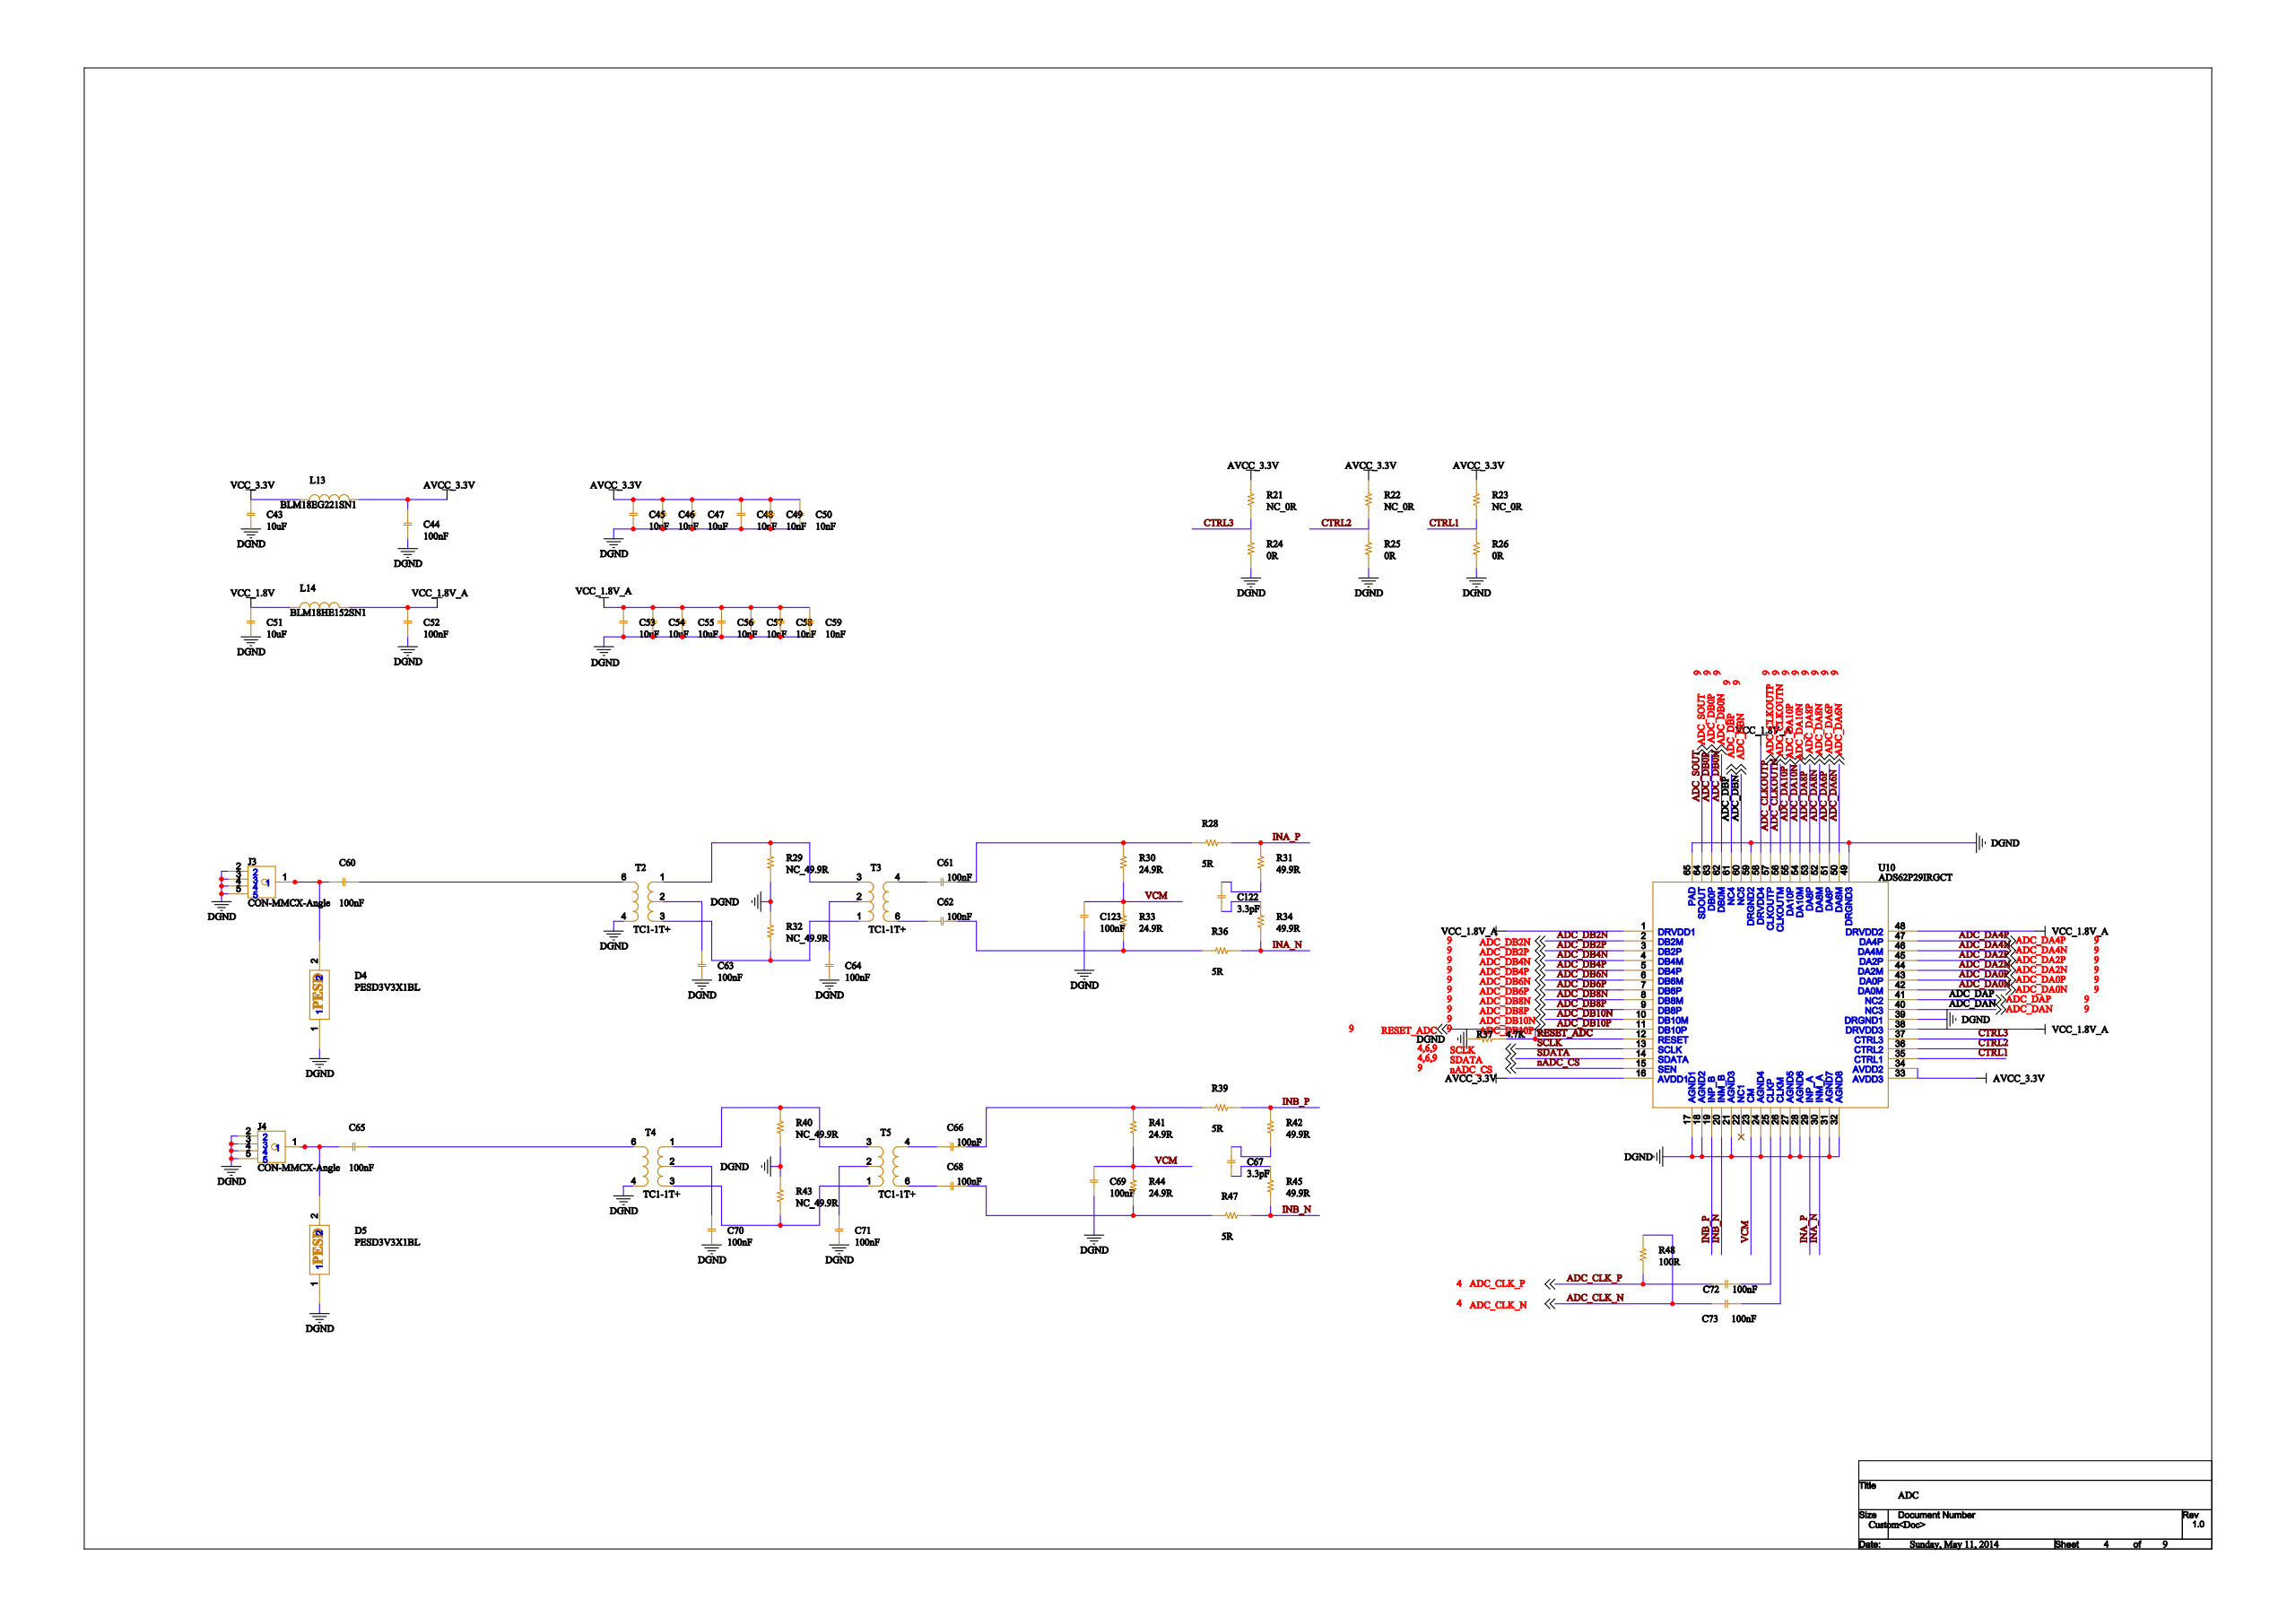Circuit board | Cadence Allegro | 233 parts | 224 nets | one sheet of the schematic
Parts on this sheet (reference | value | footprint):
C43 | 10uF | FPC-0603C
C44 | 100nF | FPC-0402C
C45 | 10uF | FPC-0603C
C46 | 10uF | FPC-0603C
C47 | 10uF | FPC-0603C
C48 | 10nF | FPC-0402C
C49 | 10nF | FPC-0402C
C50 | 10nF | FPC-0402C
C51 | 10uF | FPC-0603C
C52 | 100nF | FPC-0402C
C53 | 10uF | FPC-0603C
C54 | 10uF | FPC-0603C
C55 | 10uF | FPC-0603C
C56 | 10nF | FPC-0402C
C57 | 10nF | FPC-0402C
C58 | 10nF | FPC-0402C
C59 | 10nF | FPC-0402C
C60 | 100nF | FPC-0402C
C61 | 100nF | FPC-0402C
C62 | 100nF | FPC-0402C
C63 | 100nF | FPC-0402C
C64 | 100nF | FPC-0402C
C65 | 100nF | FPC-0402C
C66 | 100nF | FPC-0402C
C67 | 3.3pF | FPC-0402C
C68 | 100nF | FPC-0402C
C69 | 100nF | FPC-0402C
C70 | 100nF | FPC-0402C
C71 | 100nF | FPC-0402C
C72 | 100nF | FPC-0402C
C73 | 100nF | FPC-0402C
C122 | 3.3pF | FPC-0402C
C123 | 100nF | FPC-0402C
D4 | PESD3V3X1BL | SOD882
D5 | PESD3V3X1BL | SOD882
J3 | CON-MMCX-Angle | SMA
J4 | CON-MMCX-Angle | SMA
L13 | BLM18EG221SN1 | FPC-0603L
L14 | BLM18HE152SN1 | FPC-0603L
R21 | NC_0R | FPC-0603R
R22 | NC_0R | FPC-0603R
R23 | NC_0R | FPC-0603R
R24 | 0R | FPC-0603R
R25 | 0R | FPC-0603R
R26 | 0R | FPC-0603R
R28 | 5R | FPC-0402R
R29 | NC_49.9R | FPC-0603R
R30 | 24.9R | FPC-0402R
R31 | 49.9R | FPC-0402R
R32 | NC_49.9R | FPC-0603R
R33 | 24.9R | FPC-0402R
R34 | 49.9R | FPC-0402R
R36 | 5R | FPC-0402R
R37 | 4.7K | FPC-0603R
R39 | 5R | FPC-0402R
R40 | NC_49.9R | FPC-0603R
R41 | 24.9R | FPC-0402R
R42 | 49.9R | FPC-0402R
R43 | NC_49.9R | FPC-0603R
R44 | 24.9R | FPC-0402R
R45 | 49.9R | FPC-0402R
R47 | 5R | FPC-0402R
R48 | 100R | FPC-0603R
T2 | TC1-1T+ | FPC-TRAN5SM-3R81X3R81
T3 | TC1-1T+ | FPC-TRAN5SM-3R81X3R81
T4 | TC1-1T+ | FPC-TRAN5SM-3R81X3R81
T5 | TC1-1T+ | FPC-TRAN5SM-3R81X3R81
U10 | ADS62P29IRGCT | FPC-QFN9X9-64-1
Nets of these parts (net: part-pin ...):
DGND: C43-1 C44-1 C45-1 C46-1 C47-1 C48-1 C49-2 C50-1 C51-1 C52-1 C53-1 C54-1 C55-1 C56-1 C57-2 C58-2 C59-1 C63-1 C64-1 C69-1 C70-1 C71-1 C123-1 D4-1 D5-1 J3-2 J3-3 J3-4 J3-5 J4-2 J4-3 J4-4 J4-5 R24-1 R25-1 R26-1 R29-1 R32-2 R37-1 R40-1 R43-2 T2-4 T4-4 U10-17 U10-18 U10-21 U10-24 U10-27 U10-28 U10-31 U10-32 U10-39 U10-49 U10-59 U10-65
N109967: C60-1 D4-2 J3-1
N16324: C65-1 D5-2 J4-1
AVCC_3.3V: C44-2 C45-2 C46-2 C47-2 C48-2 C49-1 C50-2 L13-2 R21-2 R22-2 R23-2 U10-16 U10-33 U10-34
VCC_3.3V: C43-2 L13-1
VCM: C69-2 C123-2 R30-1 R33-2 R41-1 R44-2 U10-23
VCC_1.8V_A: C52-2 C53-2 C54-2 C55-2 C56-2 C57-1 C58-1 C59-2 L14-2 U10-1 U10-38 U10-48 U10-58
N21635: C60-2 T2-6
N109717: C61-1 T3-4
N00112: C61-2 R28-1 R30-2
N109719: C62-1 T3-6
N00118: C62-2 R33-1 R36-1
N00534: C63-2 T2-2
N109713: C64-2 T3-2
N17032: C65-2 T4-6
N16312: C66-1 T5-4
N16316: C66-2 R39-1 R41-2
N110107: C68-1 T5-6
N16420: C68-2 R44-1 R47-1
N16344: C70-2 T4-2
N16332: C71-2 T5-2
N109769: C72-1 U10-25
ADC_CLK_P: C72-2 R48-1
N00064: C73-1 U10-26
ADC_CLK_N: C73-2 R48-2
VCC_1.8V: C51-2 L14-1
N14435: C122-1 R34-2
N14423: C122-2 R31-1
N17020: C67-1 R45-2
N17008: C67-2 R42-1
ADC_CLKOUTN: U10-56
ADC_CLKOUTP: U10-57
ADC_DA4N: U10-46
ADC_DA4P: U10-47
ADC_DA0N: U10-42
ADC_DA0P: U10-43
ADC_DA6N: U10-50
ADC_DA6P: U10-51
ADC_DA2N: U10-44
ADC_DA2P: U10-45
ADC_DAN: U10-40
ADC_DAP: U10-41
ADC_DB0N: U10-62
ADC_DB0P: U10-63
ADC_DA10N: U10-54
ADC_DA10P: U10-55
ADC_DA8N: U10-52
ADC_DA8P: U10-53
ADC_DB8N: U10-8
ADC_DB8P: U10-9
ADC_DB4N: U10-4
ADC_DB4P: U10-5
ADC_DBN: U10-60
ADC_DBP: U10-61
ADC_DB6N: U10-6
ADC_DB6P: U10-7
ADC_DB10N: U10-10
ADC_DB10P: U10-11
ADC_DB2N: U10-2
ADC_DB2P: U10-3
RESET_ADC: R37-2 U10-12
CTRL3: R21-1 R24-2 U10-37
CTRL2: R22-1 R25-2 U10-36
CTRL1: R23-1 R26-2 U10-35
INA_P: R28-2 R31-2 U10-29
INA_N: R34-1 R36-2 U10-30
INB_P: R39-2 R42-2 U10-19
INB_N: R45-1 R47-2 U10-20
N13978: R29-2 T2-1 T3-3
N00070: R32-1 T2-3 T3-1
N16348: R40-2 T4-1 T5-3
N16352: R43-1 T4-3 T5-1
SCLK: U10-13
SDATA: U10-14
ADC_SOUT: U10-64